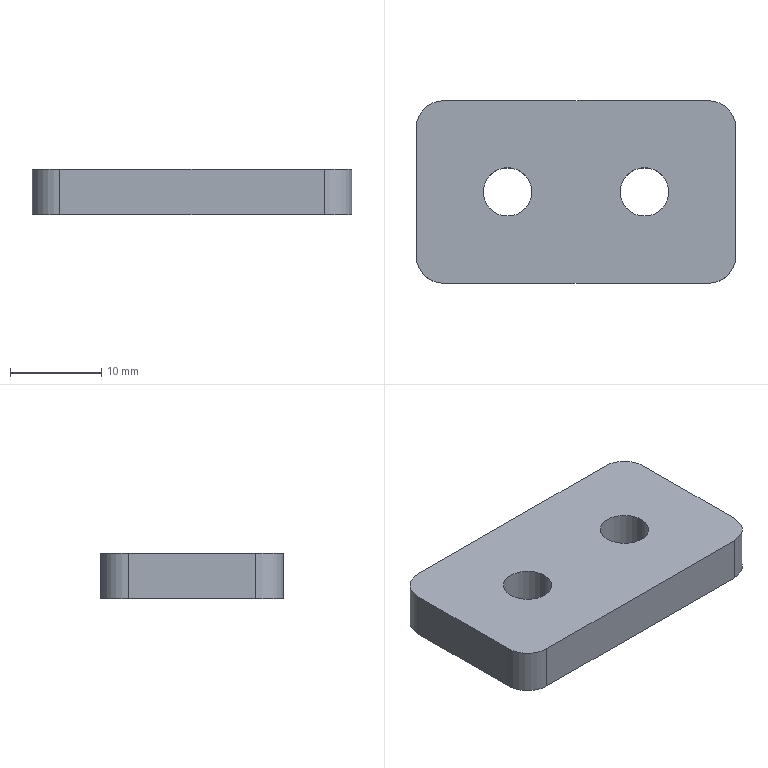Part | SolidWorks | features BaseBody 1 | 1 solid | 14 faces | box 35 x 20 x 5 mm | volume 3241 mm3 | cylinder 8 | plane 6 | commonest cylinder face diameters 5.3 x4 6 x4
STEP:
#1=CARTESIAN_POINT('',(-10.15,0.,5.));
#2=VERTEX_POINT('',#1);
#3=CARTESIAN_POINT('',(-4.85,0.,5.));
#4=VERTEX_POINT('',#3);
#5=CARTESIAN_POINT('',(-7.5,0.,5.));
#6=DIRECTION('',(0.,0.,1.));
#7=DIRECTION('',(-1.,0.,0.));
#8=AXIS2_PLACEMENT_3D('',#5,#6,#7);
#9=CIRCLE('',#8,2.65);
#10=EDGE_CURVE('',#2,#4,#9,.T.);
#11=ORIENTED_EDGE('',*,*,#10,.T.);
#12=CARTESIAN_POINT('',(-4.85,0.,0.));
#13=VERTEX_POINT('',#12);
#14=CARTESIAN_POINT('',(-4.85,0.,5.));
#15=DIRECTION('',(0.,0.,-1.));
#16=VECTOR('',#15,1000.);
#17=LINE('',#14,#16);
#18=EDGE_CURVE('',#4,#13,#17,.T.);
#19=ORIENTED_EDGE('',*,*,#18,.T.);
#20=CARTESIAN_POINT('',(-10.15,0.,0.));
#21=VERTEX_POINT('',#20);
#22=CARTESIAN_POINT('',(-7.5,0.,0.));
#23=DIRECTION('',(0.,0.,1.));
#24=DIRECTION('',(-1.,0.,0.));
#25=AXIS2_PLACEMENT_3D('',#22,#23,#24);
#26=CIRCLE('',#25,2.65);
#27=EDGE_CURVE('',#21,#13,#26,.T.);
#28=ORIENTED_EDGE('',*,*,#27,.F.);
#29=CARTESIAN_POINT('',(-10.15,0.,5.));
#30=DIRECTION('',(0.,0.,-1.));
#31=VECTOR('',#30,1000.);
#32=LINE('',#29,#31);
#33=EDGE_CURVE('',#2,#21,#32,.T.);
#34=ORIENTED_EDGE('',*,*,#33,.F.);
#35=EDGE_LOOP('',(#11,#19,#28,#34));
#36=FACE_OUTER_BOUND('',#35,.T.);
#37=CARTESIAN_POINT('',(-7.5,0.,5.));
#38=DIRECTION('',(0.,0.,-1.));
#39=DIRECTION('',(-1.,0.,0.));
#40=AXIS2_PLACEMENT_3D('',#37,#38,#39);
#41=CYLINDRICAL_SURFACE('',#40,2.65);
#42=ADVANCED_FACE('',(#36),#41,.F.);
#43=CARTESIAN_POINT('',(4.85,0.,5.));
#44=VERTEX_POINT('',#43);
#45=CARTESIAN_POINT('',(10.15,0.,5.));
#46=VERTEX_POINT('',#45);
#47=CARTESIAN_POINT('',(7.5,0.,5.));
#48=DIRECTION('',(0.,0.,1.));
#49=DIRECTION('',(-1.,0.,0.));
#50=AXIS2_PLACEMENT_3D('',#47,#48,#49);
#51=CIRCLE('',#50,2.65);
#52=EDGE_CURVE('',#44,#46,#51,.T.);
#53=ORIENTED_EDGE('',*,*,#52,.T.);
#54=CARTESIAN_POINT('',(10.15,0.,0.));
#55=VERTEX_POINT('',#54);
#56=CARTESIAN_POINT('',(10.15,0.,5.));
#57=DIRECTION('',(0.,0.,-1.));
#58=VECTOR('',#57,1000.);
#59=LINE('',#56,#58);
#60=EDGE_CURVE('',#46,#55,#59,.T.);
#61=ORIENTED_EDGE('',*,*,#60,.T.);
#62=CARTESIAN_POINT('',(4.85,0.,0.));
#63=VERTEX_POINT('',#62);
#64=CARTESIAN_POINT('',(7.5,0.,0.));
#65=DIRECTION('',(0.,0.,1.));
#66=DIRECTION('',(-1.,0.,0.));
#67=AXIS2_PLACEMENT_3D('',#64,#65,#66);
#68=CIRCLE('',#67,2.65);
#69=EDGE_CURVE('',#63,#55,#68,.T.);
#70=ORIENTED_EDGE('',*,*,#69,.F.);
#71=CARTESIAN_POINT('',(4.85,0.,5.));
#72=DIRECTION('',(0.,0.,-1.));
#73=VECTOR('',#72,1000.);
#74=LINE('',#71,#73);
#75=EDGE_CURVE('',#44,#63,#74,.T.);
#76=ORIENTED_EDGE('',*,*,#75,.F.);
#77=EDGE_LOOP('',(#53,#61,#70,#76));
#78=FACE_OUTER_BOUND('',#77,.T.);
#79=CARTESIAN_POINT('',(7.5,0.,5.));
#80=DIRECTION('',(0.,0.,-1.));
#81=DIRECTION('',(-1.,0.,0.));
#82=AXIS2_PLACEMENT_3D('',#79,#80,#81);
#83=CYLINDRICAL_SURFACE('',#82,2.65);
#84=ADVANCED_FACE('',(#78),#83,.F.);
#85=ORIENTED_EDGE('',*,*,#10,.F.);
#86=CARTESIAN_POINT('',(-7.5,0.,5.));
#87=DIRECTION('',(0.,0.,1.));
#88=DIRECTION('',(-1.,0.,0.));
#89=AXIS2_PLACEMENT_3D('',#86,#87,#88);
#90=CIRCLE('',#89,2.65);
#91=EDGE_CURVE('',#4,#2,#90,.T.);
#92=ORIENTED_EDGE('',*,*,#91,.F.);
#93=EDGE_LOOP('',(#85,#92));
#94=FACE_BOUND('',#93,.T.);
#95=ORIENTED_EDGE('',*,*,#52,.F.);
#96=CARTESIAN_POINT('',(7.5,0.,5.));
#97=DIRECTION('',(0.,0.,1.));
#98=DIRECTION('',(-1.,0.,0.));
#99=AXIS2_PLACEMENT_3D('',#96,#97,#98);
#100=CIRCLE('',#99,2.65);
#101=EDGE_CURVE('',#46,#44,#100,.T.);
#102=ORIENTED_EDGE('',*,*,#101,.F.);
#103=EDGE_LOOP('',(#95,#102));
#104=FACE_BOUND('',#103,.T.);
#105=CARTESIAN_POINT('',(17.5,-7.,5.));
#106=VERTEX_POINT('',#105);
#107=CARTESIAN_POINT('',(14.5,-10.,5.));
#108=VERTEX_POINT('',#107);
#109=CARTESIAN_POINT('',(14.5,-7.,5.));
#110=DIRECTION('',(0.,0.,-1.));
#111=DIRECTION('',(-1.,0.,0.));
#112=AXIS2_PLACEMENT_3D('',#109,#110,#111);
#113=CIRCLE('',#112,3.);
#114=EDGE_CURVE('',#106,#108,#113,.T.);
#115=ORIENTED_EDGE('',*,*,#114,.F.);
#116=CARTESIAN_POINT('',(17.5,7.,5.));
#117=VERTEX_POINT('',#116);
#118=CARTESIAN_POINT('',(17.5,0.,5.));
#119=DIRECTION('',(0.,-1.,0.));
#120=VECTOR('',#119,1000.);
#121=LINE('',#118,#120);
#122=EDGE_CURVE('',#117,#106,#121,.T.);
#123=ORIENTED_EDGE('',*,*,#122,.F.);
#124=CARTESIAN_POINT('',(14.5,10.,5.));
#125=VERTEX_POINT('',#124);
#126=CARTESIAN_POINT('',(14.5,7.,5.));
#127=DIRECTION('',(0.,0.,-1.));
#128=DIRECTION('',(-1.,0.,0.));
#129=AXIS2_PLACEMENT_3D('',#126,#127,#128);
#130=CIRCLE('',#129,3.);
#131=EDGE_CURVE('',#125,#117,#130,.T.);
#132=ORIENTED_EDGE('',*,*,#131,.F.);
#133=CARTESIAN_POINT('',(-14.5,10.,5.));
#134=VERTEX_POINT('',#133);
#135=CARTESIAN_POINT('',(0.,10.,5.));
#136=DIRECTION('',(1.,0.,0.));
#137=VECTOR('',#136,1000.);
#138=LINE('',#135,#137);
#139=EDGE_CURVE('',#134,#125,#138,.T.);
#140=ORIENTED_EDGE('',*,*,#139,.F.);
#141=CARTESIAN_POINT('',(-17.5,7.,5.));
#142=VERTEX_POINT('',#141);
#143=CARTESIAN_POINT('',(-14.5,7.,5.));
#144=DIRECTION('',(0.,0.,-1.));
#145=DIRECTION('',(-1.,0.,0.));
#146=AXIS2_PLACEMENT_3D('',#143,#144,#145);
#147=CIRCLE('',#146,3.);
#148=EDGE_CURVE('',#142,#134,#147,.T.);
#149=ORIENTED_EDGE('',*,*,#148,.F.);
#150=CARTESIAN_POINT('',(-17.5,-7.,5.));
#151=VERTEX_POINT('',#150);
#152=CARTESIAN_POINT('',(-17.5,0.,5.));
#153=DIRECTION('',(0.,1.,0.));
#154=VECTOR('',#153,1000.);
#155=LINE('',#152,#154);
#156=EDGE_CURVE('',#151,#142,#155,.T.);
#157=ORIENTED_EDGE('',*,*,#156,.F.);
#158=CARTESIAN_POINT('',(-14.5,-10.,5.));
#159=VERTEX_POINT('',#158);
#160=CARTESIAN_POINT('',(-14.5,-7.,5.));
#161=DIRECTION('',(0.,0.,-1.));
#162=DIRECTION('',(-1.,0.,0.));
#163=AXIS2_PLACEMENT_3D('',#160,#161,#162);
#164=CIRCLE('',#163,3.);
#165=EDGE_CURVE('',#159,#151,#164,.T.);
#166=ORIENTED_EDGE('',*,*,#165,.F.);
#167=CARTESIAN_POINT('',(0.,-10.,5.));
#168=DIRECTION('',(-1.,0.,0.));
#169=VECTOR('',#168,1000.);
#170=LINE('',#167,#169);
#171=EDGE_CURVE('',#108,#159,#170,.T.);
#172=ORIENTED_EDGE('',*,*,#171,.F.);
#173=EDGE_LOOP('',(#115,#123,#132,#140,#149,#157,#166,#172));
#174=FACE_OUTER_BOUND('',#173,.T.);
#175=CARTESIAN_POINT('',(0.,0.,5.));
#176=DIRECTION('',(0.,0.,-1.));
#177=DIRECTION('',(-1.,0.,0.));
#178=AXIS2_PLACEMENT_3D('',#175,#176,#177);
#179=PLANE('',#178);
#180=ADVANCED_FACE('',(#94,#104,#174),#179,.F.);
#181=ORIENTED_EDGE('',*,*,#18,.F.);
#182=ORIENTED_EDGE('',*,*,#91,.T.);
#183=ORIENTED_EDGE('',*,*,#33,.T.);
#184=CARTESIAN_POINT('',(-7.5,0.,0.));
#185=DIRECTION('',(0.,0.,1.));
#186=DIRECTION('',(-1.,0.,0.));
#187=AXIS2_PLACEMENT_3D('',#184,#185,#186);
#188=CIRCLE('',#187,2.65);
#189=EDGE_CURVE('',#13,#21,#188,.T.);
#190=ORIENTED_EDGE('',*,*,#189,.F.);
#191=EDGE_LOOP('',(#181,#182,#183,#190));
#192=FACE_OUTER_BOUND('',#191,.T.);
#193=CARTESIAN_POINT('',(-7.5,0.,5.));
#194=DIRECTION('',(0.,0.,-1.));
#195=DIRECTION('',(-1.,0.,0.));
#196=AXIS2_PLACEMENT_3D('',#193,#194,#195);
#197=CYLINDRICAL_SURFACE('',#196,2.65);
#198=ADVANCED_FACE('',(#192),#197,.F.);
#199=ORIENTED_EDGE('',*,*,#60,.F.);
#200=ORIENTED_EDGE('',*,*,#101,.T.);
#201=ORIENTED_EDGE('',*,*,#75,.T.);
#202=CARTESIAN_POINT('',(7.5,0.,0.));
#203=DIRECTION('',(0.,0.,1.));
#204=DIRECTION('',(-1.,0.,0.));
#205=AXIS2_PLACEMENT_3D('',#202,#203,#204);
#206=CIRCLE('',#205,2.65);
#207=EDGE_CURVE('',#55,#63,#206,.T.);
#208=ORIENTED_EDGE('',*,*,#207,.F.);
#209=EDGE_LOOP('',(#199,#200,#201,#208));
#210=FACE_OUTER_BOUND('',#209,.T.);
#211=CARTESIAN_POINT('',(7.5,0.,5.));
#212=DIRECTION('',(0.,0.,-1.));
#213=DIRECTION('',(-1.,0.,0.));
#214=AXIS2_PLACEMENT_3D('',#211,#212,#213);
#215=CYLINDRICAL_SURFACE('',#214,2.65);
#216=ADVANCED_FACE('',(#210),#215,.F.);
#217=CARTESIAN_POINT('',(14.5,-10.,0.));
#218=VERTEX_POINT('',#217);
#219=CARTESIAN_POINT('',(14.5,-10.,5.));
#220=DIRECTION('',(0.,0.,-1.));
#221=VECTOR('',#220,1000.);
#222=LINE('',#219,#221);
#223=EDGE_CURVE('',#108,#218,#222,.T.);
#224=ORIENTED_EDGE('',*,*,#223,.F.);
#225=ORIENTED_EDGE('',*,*,#171,.T.);
#226=CARTESIAN_POINT('',(-14.5,-10.,0.));
#227=VERTEX_POINT('',#226);
#228=CARTESIAN_POINT('',(-14.5,-10.,5.));
#229=DIRECTION('',(0.,0.,1.));
#230=VECTOR('',#229,1000.);
#231=LINE('',#228,#230);
#232=EDGE_CURVE('',#227,#159,#231,.T.);
#233=ORIENTED_EDGE('',*,*,#232,.F.);
#234=CARTESIAN_POINT('',(-17.5,-10.,0.));
#235=DIRECTION('',(-1.,0.,0.));
#236=VECTOR('',#235,1000.);
#237=LINE('',#234,#236);
#238=EDGE_CURVE('',#218,#227,#237,.T.);
#239=ORIENTED_EDGE('',*,*,#238,.F.);
#240=EDGE_LOOP('',(#224,#225,#233,#239));
#241=FACE_OUTER_BOUND('',#240,.T.);
#242=CARTESIAN_POINT('',(-17.5,-10.,5.));
#243=DIRECTION('',(0.,1.,0.));
#244=DIRECTION('',(0.,0.,1.));
#245=AXIS2_PLACEMENT_3D('',#242,#243,#244);
#246=PLANE('',#245);
#247=ADVANCED_FACE('',(#241),#246,.F.);
#248=CARTESIAN_POINT('',(17.5,-7.,0.));
#249=VERTEX_POINT('',#248);
#250=CARTESIAN_POINT('',(14.5,-7.,0.));
#251=DIRECTION('',(0.,0.,1.));
#252=DIRECTION('',(-1.,0.,0.));
#253=AXIS2_PLACEMENT_3D('',#250,#251,#252);
#254=CIRCLE('',#253,3.);
#255=EDGE_CURVE('',#218,#249,#254,.T.);
#256=ORIENTED_EDGE('',*,*,#255,.T.);
#257=CARTESIAN_POINT('',(17.5,-7.,5.));
#258=DIRECTION('',(0.,0.,1.));
#259=VECTOR('',#258,1000.);
#260=LINE('',#257,#259);
#261=EDGE_CURVE('',#249,#106,#260,.T.);
#262=ORIENTED_EDGE('',*,*,#261,.T.);
#263=ORIENTED_EDGE('',*,*,#114,.T.);
#264=ORIENTED_EDGE('',*,*,#223,.T.);
#265=EDGE_LOOP('',(#256,#262,#263,#264));
#266=FACE_OUTER_BOUND('',#265,.T.);
#267=CARTESIAN_POINT('',(14.5,-7.,5.));
#268=DIRECTION('',(0.,0.,-1.));
#269=DIRECTION('',(-1.,0.,0.));
#270=AXIS2_PLACEMENT_3D('',#267,#268,#269);
#271=CYLINDRICAL_SURFACE('',#270,3.);
#272=ADVANCED_FACE('',(#266),#271,.T.);
#273=ORIENTED_EDGE('',*,*,#261,.F.);
#274=CARTESIAN_POINT('',(17.5,7.,0.));
#275=VERTEX_POINT('',#274);
#276=CARTESIAN_POINT('',(17.5,-10.,0.));
#277=DIRECTION('',(0.,-1.,0.));
#278=VECTOR('',#277,1000.);
#279=LINE('',#276,#278);
#280=EDGE_CURVE('',#275,#249,#279,.T.);
#281=ORIENTED_EDGE('',*,*,#280,.F.);
#282=CARTESIAN_POINT('',(17.5,7.,5.));
#283=DIRECTION('',(0.,0.,-1.));
#284=VECTOR('',#283,1000.);
#285=LINE('',#282,#284);
#286=EDGE_CURVE('',#117,#275,#285,.T.);
#287=ORIENTED_EDGE('',*,*,#286,.F.);
#288=ORIENTED_EDGE('',*,*,#122,.T.);
#289=EDGE_LOOP('',(#273,#281,#287,#288));
#290=FACE_OUTER_BOUND('',#289,.T.);
#291=CARTESIAN_POINT('',(17.5,-10.,5.));
#292=DIRECTION('',(-1.,0.,0.));
#293=DIRECTION('',(0.,0.,1.));
#294=AXIS2_PLACEMENT_3D('',#291,#292,#293);
#295=PLANE('',#294);
#296=ADVANCED_FACE('',(#290),#295,.F.);
#297=CARTESIAN_POINT('',(14.5,10.,0.));
#298=VERTEX_POINT('',#297);
#299=CARTESIAN_POINT('',(14.5,7.,0.));
#300=DIRECTION('',(0.,0.,1.));
#301=DIRECTION('',(-1.,0.,0.));
#302=AXIS2_PLACEMENT_3D('',#299,#300,#301);
#303=CIRCLE('',#302,3.);
#304=EDGE_CURVE('',#275,#298,#303,.T.);
#305=ORIENTED_EDGE('',*,*,#304,.T.);
#306=CARTESIAN_POINT('',(14.5,10.,5.));
#307=DIRECTION('',(0.,0.,1.));
#308=VECTOR('',#307,1000.);
#309=LINE('',#306,#308);
#310=EDGE_CURVE('',#298,#125,#309,.T.);
#311=ORIENTED_EDGE('',*,*,#310,.T.);
#312=ORIENTED_EDGE('',*,*,#131,.T.);
#313=ORIENTED_EDGE('',*,*,#286,.T.);
#314=EDGE_LOOP('',(#305,#311,#312,#313));
#315=FACE_OUTER_BOUND('',#314,.T.);
#316=CARTESIAN_POINT('',(14.5,7.,5.));
#317=DIRECTION('',(0.,0.,-1.));
#318=DIRECTION('',(-1.,0.,0.));
#319=AXIS2_PLACEMENT_3D('',#316,#317,#318);
#320=CYLINDRICAL_SURFACE('',#319,3.);
#321=ADVANCED_FACE('',(#315),#320,.T.);
#322=CARTESIAN_POINT('',(-14.5,10.,0.));
#323=VERTEX_POINT('',#322);
#324=CARTESIAN_POINT('',(-14.5,10.,5.));
#325=DIRECTION('',(0.,0.,-1.));
#326=VECTOR('',#325,1000.);
#327=LINE('',#324,#326);
#328=EDGE_CURVE('',#134,#323,#327,.T.);
#329=ORIENTED_EDGE('',*,*,#328,.F.);
#330=ORIENTED_EDGE('',*,*,#139,.T.);
#331=ORIENTED_EDGE('',*,*,#310,.F.);
#332=CARTESIAN_POINT('',(-17.5,10.,0.));
#333=DIRECTION('',(1.,0.,0.));
#334=VECTOR('',#333,1000.);
#335=LINE('',#332,#334);
#336=EDGE_CURVE('',#323,#298,#335,.T.);
#337=ORIENTED_EDGE('',*,*,#336,.F.);
#338=EDGE_LOOP('',(#329,#330,#331,#337));
#339=FACE_OUTER_BOUND('',#338,.T.);
#340=CARTESIAN_POINT('',(-17.5,10.,5.));
#341=DIRECTION('',(0.,-1.,0.));
#342=DIRECTION('',(0.,0.,-1.));
#343=AXIS2_PLACEMENT_3D('',#340,#341,#342);
#344=PLANE('',#343);
#345=ADVANCED_FACE('',(#339),#344,.F.);
#346=CARTESIAN_POINT('',(-17.5,7.,0.));
#347=VERTEX_POINT('',#346);
#348=CARTESIAN_POINT('',(-14.5,7.,0.));
#349=DIRECTION('',(0.,0.,1.));
#350=DIRECTION('',(-1.,0.,0.));
#351=AXIS2_PLACEMENT_3D('',#348,#349,#350);
#352=CIRCLE('',#351,3.);
#353=EDGE_CURVE('',#323,#347,#352,.T.);
#354=ORIENTED_EDGE('',*,*,#353,.T.);
#355=CARTESIAN_POINT('',(-17.5,7.,5.));
#356=DIRECTION('',(0.,0.,1.));
#357=VECTOR('',#356,1000.);
#358=LINE('',#355,#357);
#359=EDGE_CURVE('',#347,#142,#358,.T.);
#360=ORIENTED_EDGE('',*,*,#359,.T.);
#361=ORIENTED_EDGE('',*,*,#148,.T.);
#362=ORIENTED_EDGE('',*,*,#328,.T.);
#363=EDGE_LOOP('',(#354,#360,#361,#362));
#364=FACE_OUTER_BOUND('',#363,.T.);
#365=CARTESIAN_POINT('',(-14.5,7.,5.));
#366=DIRECTION('',(0.,0.,-1.));
#367=DIRECTION('',(-1.,0.,0.));
#368=AXIS2_PLACEMENT_3D('',#365,#366,#367);
#369=CYLINDRICAL_SURFACE('',#368,3.);
#370=ADVANCED_FACE('',(#364),#369,.T.);
#371=CARTESIAN_POINT('',(-17.5,-7.,0.));
#372=VERTEX_POINT('',#371);
#373=CARTESIAN_POINT('',(-17.5,-7.,5.));
#374=DIRECTION('',(0.,0.,-1.));
#375=VECTOR('',#374,1000.);
#376=LINE('',#373,#375);
#377=EDGE_CURVE('',#151,#372,#376,.T.);
#378=ORIENTED_EDGE('',*,*,#377,.F.);
#379=ORIENTED_EDGE('',*,*,#156,.T.);
#380=ORIENTED_EDGE('',*,*,#359,.F.);
#381=CARTESIAN_POINT('',(-17.5,-10.,0.));
#382=DIRECTION('',(0.,1.,0.));
#383=VECTOR('',#382,1000.);
#384=LINE('',#381,#383);
#385=EDGE_CURVE('',#372,#347,#384,.T.);
#386=ORIENTED_EDGE('',*,*,#385,.F.);
#387=EDGE_LOOP('',(#378,#379,#380,#386));
#388=FACE_OUTER_BOUND('',#387,.T.);
#389=CARTESIAN_POINT('',(-17.5,-10.,5.));
#390=DIRECTION('',(1.,0.,0.));
#391=DIRECTION('',(0.,0.,-1.));
#392=AXIS2_PLACEMENT_3D('',#389,#390,#391);
#393=PLANE('',#392);
#394=ADVANCED_FACE('',(#388),#393,.F.);
#395=CARTESIAN_POINT('',(-14.5,-7.,0.));
#396=DIRECTION('',(0.,0.,1.));
#397=DIRECTION('',(-1.,0.,0.));
#398=AXIS2_PLACEMENT_3D('',#395,#396,#397);
#399=CIRCLE('',#398,3.);
#400=EDGE_CURVE('',#372,#227,#399,.T.);
#401=ORIENTED_EDGE('',*,*,#400,.T.);
#402=ORIENTED_EDGE('',*,*,#232,.T.);
#403=ORIENTED_EDGE('',*,*,#165,.T.);
#404=ORIENTED_EDGE('',*,*,#377,.T.);
#405=EDGE_LOOP('',(#401,#402,#403,#404));
#406=FACE_OUTER_BOUND('',#405,.T.);
#407=CARTESIAN_POINT('',(-14.5,-7.,5.));
#408=DIRECTION('',(0.,0.,-1.));
#409=DIRECTION('',(-1.,0.,0.));
#410=AXIS2_PLACEMENT_3D('',#407,#408,#409);
#411=CYLINDRICAL_SURFACE('',#410,3.);
#412=ADVANCED_FACE('',(#406),#411,.T.);
#413=ORIENTED_EDGE('',*,*,#27,.T.);
#414=ORIENTED_EDGE('',*,*,#189,.T.);
#415=EDGE_LOOP('',(#413,#414));
#416=FACE_BOUND('',#415,.T.);
#417=ORIENTED_EDGE('',*,*,#336,.T.);
#418=ORIENTED_EDGE('',*,*,#304,.F.);
#419=ORIENTED_EDGE('',*,*,#280,.T.);
#420=ORIENTED_EDGE('',*,*,#255,.F.);
#421=ORIENTED_EDGE('',*,*,#238,.T.);
#422=ORIENTED_EDGE('',*,*,#400,.F.);
#423=ORIENTED_EDGE('',*,*,#385,.T.);
#424=ORIENTED_EDGE('',*,*,#353,.F.);
#425=EDGE_LOOP('',(#417,#418,#419,#420,#421,#422,#423,#424));
#426=FACE_OUTER_BOUND('',#425,.T.);
#427=ORIENTED_EDGE('',*,*,#69,.T.);
#428=ORIENTED_EDGE('',*,*,#207,.T.);
#429=EDGE_LOOP('',(#427,#428));
#430=FACE_BOUND('',#429,.T.);
#431=CARTESIAN_POINT('',(0.,0.,0.));
#432=DIRECTION('',(0.,0.,-1.));
#433=DIRECTION('',(-1.,0.,0.));
#434=AXIS2_PLACEMENT_3D('',#431,#432,#433);
#435=PLANE('',#434);
#436=ADVANCED_FACE('',(#416,#426,#430),#435,.T.);
#437=CLOSED_SHELL('',(#42,#84,#180,#198,#216,#247,#272,#296,#321,#345,#370,#394,#412,#436));
#438=MANIFOLD_SOLID_BREP('',#437);
#439=CARTESIAN_POINT('',(0.,0.,0.));
#440=DIRECTION('',(0.,0.,1.));
#441=DIRECTION('',(1.,0.,0.));
#442=AXIS2_PLACEMENT_3D('',#439,#440,#441);
#443=(LENGTH_UNIT()NAMED_UNIT(*)SI_UNIT(.MILLI.,.METRE.));
#444=UNCERTAINTY_MEASURE_WITH_UNIT(LENGTH_MEASURE(0.00001),#443,'','');
#445=(NAMED_UNIT(*)PLANE_ANGLE_UNIT()SI_UNIT($,.RADIAN.));
#446=(NAMED_UNIT(*)SI_UNIT($,.STERADIAN.)SOLID_ANGLE_UNIT());
#447=(GEOMETRIC_REPRESENTATION_CONTEXT(3)GLOBAL_UNCERTAINTY_ASSIGNED_CONTEXT((#444))GLOBAL_UNIT_ASSIGNED_CONTEXT((#443,#445,#446))REPRESENTATION_CONTEXT('',''));
#448=ADVANCED_BREP_SHAPE_REPRESENTATION('',(#438,#442),#447);